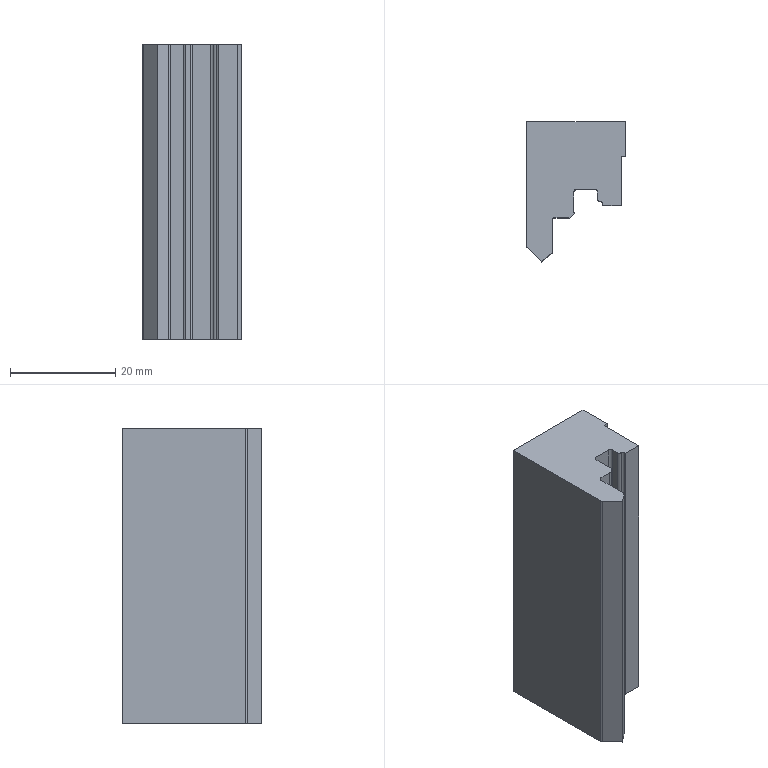Part | NX | features BREP 2 | 2 solids | 54 faces | box 18.792 x 26.496 x 56 mm | volume 37129 mm3 | plane 34 | cylinder 20 | commonest cylinder face diameters 1 x20